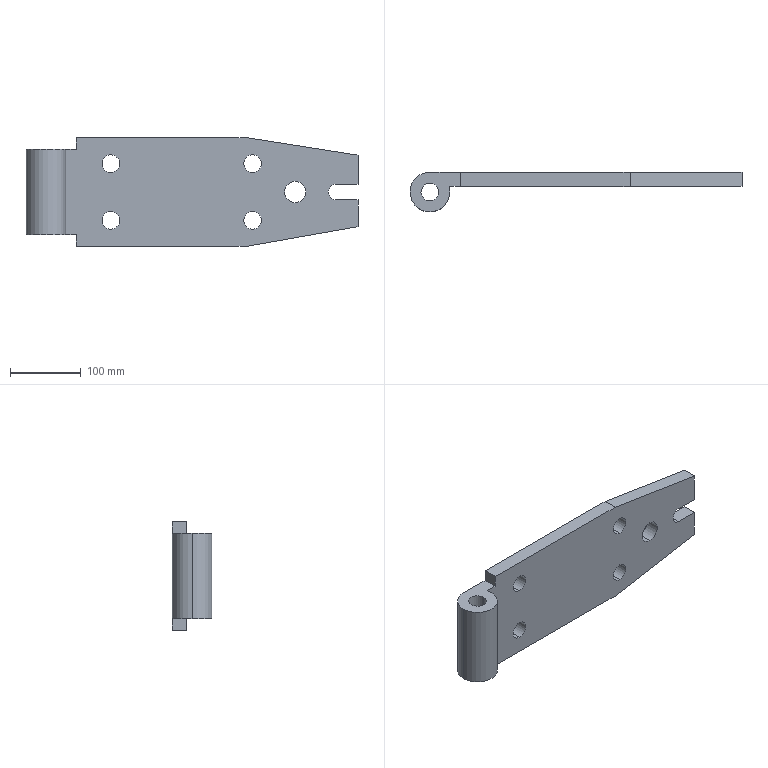Part | SolidWorks | features Extrusion 1, ICE 1 | 1 solid | 30 faces | box 468.278 x 56 x 153.374 mm | volume 1357843 mm3 | cylinder 15 | plane 15 | commonest cylinder face diameters 25 x10 30 x2 56 x2 22.074 x1
STEP:
#1=CARTESIAN_POINT('',(-212.267,-8.,60.));
#2=VERTEX_POINT('',#1);
#3=CARTESIAN_POINT('',(-187.267,-8.,60.));
#4=VERTEX_POINT('',#3);
#5=CARTESIAN_POINT('',(-199.767,-8.,60.));
#6=DIRECTION('',(0.,0.,1.));
#7=DIRECTION('',(1.,0.,0.));
#8=AXIS2_PLACEMENT_3D('',#5,#6,#7);
#9=CIRCLE('',#8,12.5);
#10=EDGE_CURVE('',#2,#4,#9,.T.);
#11=ORIENTED_EDGE('',*,*,#10,.T.);
#12=CARTESIAN_POINT('',(-187.267,-8.,-60.));
#13=VERTEX_POINT('',#12);
#14=CARTESIAN_POINT('',(-187.267,-8.,60.));
#15=DIRECTION('',(0.,0.,-1.));
#16=VECTOR('',#15,1000.);
#17=LINE('',#14,#16);
#18=EDGE_CURVE('',#4,#13,#17,.T.);
#19=ORIENTED_EDGE('',*,*,#18,.T.);
#20=CARTESIAN_POINT('',(-212.267,-8.,-60.));
#21=VERTEX_POINT('',#20);
#22=CARTESIAN_POINT('',(-199.767,-8.,-60.));
#23=DIRECTION('',(0.,0.,1.));
#24=DIRECTION('',(1.,0.,0.));
#25=AXIS2_PLACEMENT_3D('',#22,#23,#24);
#26=CIRCLE('',#25,12.5);
#27=EDGE_CURVE('',#21,#13,#26,.T.);
#28=ORIENTED_EDGE('',*,*,#27,.F.);
#29=CARTESIAN_POINT('',(-212.267,-8.,60.));
#30=DIRECTION('',(0.,0.,-1.));
#31=VECTOR('',#30,1000.);
#32=LINE('',#29,#31);
#33=EDGE_CURVE('',#2,#21,#32,.T.);
#34=ORIENTED_EDGE('',*,*,#33,.F.);
#35=EDGE_LOOP('',(#11,#19,#28,#34));
#36=FACE_OUTER_BOUND('',#35,.T.);
#37=CARTESIAN_POINT('',(-199.767,-8.,60.));
#38=DIRECTION('',(0.,0.,-1.));
#39=DIRECTION('',(-1.,0.,0.));
#40=AXIS2_PLACEMENT_3D('',#37,#38,#39);
#41=CYLINDRICAL_SURFACE('',#40,12.5);
#42=ADVANCED_FACE('',(#36),#41,.F.);
#43=CARTESIAN_POINT('',(-227.767,-8.,60.));
#44=VERTEX_POINT('',#43);
#45=CARTESIAN_POINT('',(-171.767,-8.,60.));
#46=VERTEX_POINT('',#45);
#47=CARTESIAN_POINT('',(-199.767,-8.,60.));
#48=DIRECTION('',(0.,0.,1.));
#49=DIRECTION('',(1.,0.,0.));
#50=AXIS2_PLACEMENT_3D('',#47,#48,#49);
#51=CIRCLE('',#50,28.);
#52=EDGE_CURVE('',#44,#46,#51,.T.);
#53=ORIENTED_EDGE('',*,*,#52,.F.);
#54=CARTESIAN_POINT('',(-227.767,-8.,-60.));
#55=VERTEX_POINT('',#54);
#56=CARTESIAN_POINT('',(-227.767,-8.,60.));
#57=DIRECTION('',(0.,0.,-1.));
#58=VECTOR('',#57,1000.);
#59=LINE('',#56,#58);
#60=EDGE_CURVE('',#44,#55,#59,.T.);
#61=ORIENTED_EDGE('',*,*,#60,.T.);
#62=CARTESIAN_POINT('',(-171.767,-8.,-60.));
#63=VERTEX_POINT('',#62);
#64=CARTESIAN_POINT('',(-199.767,-8.,-60.));
#65=DIRECTION('',(0.,0.,1.));
#66=DIRECTION('',(1.,0.,0.));
#67=AXIS2_PLACEMENT_3D('',#64,#65,#66);
#68=CIRCLE('',#67,28.);
#69=EDGE_CURVE('',#55,#63,#68,.T.);
#70=ORIENTED_EDGE('',*,*,#69,.T.);
#71=CARTESIAN_POINT('',(-171.767,-8.,60.));
#72=DIRECTION('',(0.,0.,-1.));
#73=VECTOR('',#72,1000.);
#74=LINE('',#71,#73);
#75=EDGE_CURVE('',#46,#63,#74,.T.);
#76=ORIENTED_EDGE('',*,*,#75,.F.);
#77=EDGE_LOOP('',(#53,#61,#70,#76));
#78=FACE_OUTER_BOUND('',#77,.T.);
#79=CARTESIAN_POINT('',(-199.767,-8.,60.));
#80=DIRECTION('',(0.,0.,-1.));
#81=DIRECTION('',(-1.,0.,0.));
#82=AXIS2_PLACEMENT_3D('',#79,#80,#81);
#83=CYLINDRICAL_SURFACE('',#82,28.);
#84=ADVANCED_FACE('',(#78),#83,.T.);
#85=CARTESIAN_POINT('',(-108.15,20.,27.5));
#86=VERTEX_POINT('',#85);
#87=CARTESIAN_POINT('',(-108.15,20.,52.5));
#88=VERTEX_POINT('',#87);
#89=CARTESIAN_POINT('',(-108.15,20.,40.));
#90=DIRECTION('',(0.,1.,0.));
#91=DIRECTION('',(0.,0.,1.));
#92=AXIS2_PLACEMENT_3D('',#89,#90,#91);
#93=CIRCLE('',#92,12.5);
#94=EDGE_CURVE('',#86,#88,#93,.T.);
#95=ORIENTED_EDGE('',*,*,#94,.T.);
#96=CARTESIAN_POINT('',(-108.15,0.,52.5));
#97=VERTEX_POINT('',#96);
#98=CARTESIAN_POINT('',(-108.15,20.,52.5));
#99=DIRECTION('',(0.,-1.,0.));
#100=VECTOR('',#99,1000.);
#101=LINE('',#98,#100);
#102=EDGE_CURVE('',#88,#97,#101,.T.);
#103=ORIENTED_EDGE('',*,*,#102,.T.);
#104=CARTESIAN_POINT('',(-108.15,0.,27.5));
#105=VERTEX_POINT('',#104);
#106=CARTESIAN_POINT('',(-108.15,0.,40.));
#107=DIRECTION('',(0.,1.,0.));
#108=DIRECTION('',(0.,0.,1.));
#109=AXIS2_PLACEMENT_3D('',#106,#107,#108);
#110=CIRCLE('',#109,12.5);
#111=EDGE_CURVE('',#105,#97,#110,.T.);
#112=ORIENTED_EDGE('',*,*,#111,.F.);
#113=CARTESIAN_POINT('',(-108.15,20.,27.5));
#114=DIRECTION('',(0.,-1.,0.));
#115=VECTOR('',#114,1000.);
#116=LINE('',#113,#115);
#117=EDGE_CURVE('',#86,#105,#116,.T.);
#118=ORIENTED_EDGE('',*,*,#117,.F.);
#119=EDGE_LOOP('',(#95,#103,#112,#118));
#120=FACE_OUTER_BOUND('',#119,.T.);
#121=CARTESIAN_POINT('',(-108.15,20.,40.));
#122=DIRECTION('',(0.,-1.,0.));
#123=DIRECTION('',(0.,0.,-1.));
#124=AXIS2_PLACEMENT_3D('',#121,#122,#123);
#125=CYLINDRICAL_SURFACE('',#124,12.5);
#126=ADVANCED_FACE('',(#120),#125,.F.);
#127=CARTESIAN_POINT('',(91.85,20.,27.5));
#128=VERTEX_POINT('',#127);
#129=CARTESIAN_POINT('',(91.85,20.,52.5));
#130=VERTEX_POINT('',#129);
#131=CARTESIAN_POINT('',(91.85,20.,40.));
#132=DIRECTION('',(0.,1.,0.));
#133=DIRECTION('',(0.,0.,1.));
#134=AXIS2_PLACEMENT_3D('',#131,#132,#133);
#135=CIRCLE('',#134,12.5);
#136=EDGE_CURVE('',#128,#130,#135,.T.);
#137=ORIENTED_EDGE('',*,*,#136,.T.);
#138=CARTESIAN_POINT('',(91.85,0.,52.5));
#139=VERTEX_POINT('',#138);
#140=CARTESIAN_POINT('',(91.85,20.,52.5));
#141=DIRECTION('',(0.,-1.,0.));
#142=VECTOR('',#141,1000.);
#143=LINE('',#140,#142);
#144=EDGE_CURVE('',#130,#139,#143,.T.);
#145=ORIENTED_EDGE('',*,*,#144,.T.);
#146=CARTESIAN_POINT('',(91.85,0.,27.5));
#147=VERTEX_POINT('',#146);
#148=CARTESIAN_POINT('',(91.85,0.,40.));
#149=DIRECTION('',(0.,1.,0.));
#150=DIRECTION('',(0.,0.,1.));
#151=AXIS2_PLACEMENT_3D('',#148,#149,#150);
#152=CIRCLE('',#151,12.5);
#153=EDGE_CURVE('',#147,#139,#152,.T.);
#154=ORIENTED_EDGE('',*,*,#153,.F.);
#155=CARTESIAN_POINT('',(91.85,20.,27.5));
#156=DIRECTION('',(0.,-1.,0.));
#157=VECTOR('',#156,1000.);
#158=LINE('',#155,#157);
#159=EDGE_CURVE('',#128,#147,#158,.T.);
#160=ORIENTED_EDGE('',*,*,#159,.F.);
#161=EDGE_LOOP('',(#137,#145,#154,#160));
#162=FACE_OUTER_BOUND('',#161,.T.);
#163=CARTESIAN_POINT('',(91.85,20.,40.));
#164=DIRECTION('',(0.,-1.,0.));
#165=DIRECTION('',(0.,0.,-1.));
#166=AXIS2_PLACEMENT_3D('',#163,#164,#165);
#167=CYLINDRICAL_SURFACE('',#166,12.5);
#168=ADVANCED_FACE('',(#162),#167,.F.);
#169=CARTESIAN_POINT('',(151.85,20.,-15.));
#170=VERTEX_POINT('',#169);
#171=CARTESIAN_POINT('',(151.85,20.,15.));
#172=VERTEX_POINT('',#171);
#173=CARTESIAN_POINT('',(151.85,20.,0.));
#174=DIRECTION('',(0.,1.,0.));
#175=DIRECTION('',(0.,0.,1.));
#176=AXIS2_PLACEMENT_3D('',#173,#174,#175);
#177=CIRCLE('',#176,15.);
#178=EDGE_CURVE('',#170,#172,#177,.T.);
#179=ORIENTED_EDGE('',*,*,#178,.T.);
#180=CARTESIAN_POINT('',(151.85,0.,15.));
#181=VERTEX_POINT('',#180);
#182=CARTESIAN_POINT('',(151.85,20.,15.));
#183=DIRECTION('',(0.,-1.,0.));
#184=VECTOR('',#183,1000.);
#185=LINE('',#182,#184);
#186=EDGE_CURVE('',#172,#181,#185,.T.);
#187=ORIENTED_EDGE('',*,*,#186,.T.);
#188=CARTESIAN_POINT('',(151.85,0.,-15.));
#189=VERTEX_POINT('',#188);
#190=CARTESIAN_POINT('',(151.85,0.,0.));
#191=DIRECTION('',(0.,1.,0.));
#192=DIRECTION('',(0.,0.,1.));
#193=AXIS2_PLACEMENT_3D('',#190,#191,#192);
#194=CIRCLE('',#193,15.);
#195=EDGE_CURVE('',#189,#181,#194,.T.);
#196=ORIENTED_EDGE('',*,*,#195,.F.);
#197=CARTESIAN_POINT('',(151.85,20.,-15.));
#198=DIRECTION('',(0.,-1.,0.));
#199=VECTOR('',#198,1000.);
#200=LINE('',#197,#199);
#201=EDGE_CURVE('',#170,#189,#200,.T.);
#202=ORIENTED_EDGE('',*,*,#201,.F.);
#203=EDGE_LOOP('',(#179,#187,#196,#202));
#204=FACE_OUTER_BOUND('',#203,.T.);
#205=CARTESIAN_POINT('',(151.85,20.,0.));
#206=DIRECTION('',(0.,-1.,0.));
#207=DIRECTION('',(0.,0.,-1.));
#208=AXIS2_PLACEMENT_3D('',#205,#206,#207);
#209=CYLINDRICAL_SURFACE('',#208,15.);
#210=ADVANCED_FACE('',(#204),#209,.F.);
#211=CARTESIAN_POINT('',(-108.15,20.,-52.5));
#212=VERTEX_POINT('',#211);
#213=CARTESIAN_POINT('',(-108.15,20.,-27.5));
#214=VERTEX_POINT('',#213);
#215=CARTESIAN_POINT('',(-108.15,20.,-40.));
#216=DIRECTION('',(0.,1.,0.));
#217=DIRECTION('',(0.,0.,1.));
#218=AXIS2_PLACEMENT_3D('',#215,#216,#217);
#219=CIRCLE('',#218,12.5);
#220=EDGE_CURVE('',#212,#214,#219,.T.);
#221=ORIENTED_EDGE('',*,*,#220,.T.);
#222=CARTESIAN_POINT('',(-108.15,0.,-27.5));
#223=VERTEX_POINT('',#222);
#224=CARTESIAN_POINT('',(-108.15,20.,-27.5));
#225=DIRECTION('',(0.,-1.,0.));
#226=VECTOR('',#225,1000.);
#227=LINE('',#224,#226);
#228=EDGE_CURVE('',#214,#223,#227,.T.);
#229=ORIENTED_EDGE('',*,*,#228,.T.);
#230=CARTESIAN_POINT('',(-108.15,0.,-52.5));
#231=VERTEX_POINT('',#230);
#232=CARTESIAN_POINT('',(-108.15,0.,-40.));
#233=DIRECTION('',(0.,1.,0.));
#234=DIRECTION('',(0.,0.,1.));
#235=AXIS2_PLACEMENT_3D('',#232,#233,#234);
#236=CIRCLE('',#235,12.5);
#237=EDGE_CURVE('',#231,#223,#236,.T.);
#238=ORIENTED_EDGE('',*,*,#237,.F.);
#239=CARTESIAN_POINT('',(-108.15,20.,-52.5));
#240=DIRECTION('',(0.,-1.,0.));
#241=VECTOR('',#240,1000.);
#242=LINE('',#239,#241);
#243=EDGE_CURVE('',#212,#231,#242,.T.);
#244=ORIENTED_EDGE('',*,*,#243,.F.);
#245=EDGE_LOOP('',(#221,#229,#238,#244));
#246=FACE_OUTER_BOUND('',#245,.T.);
#247=CARTESIAN_POINT('',(-108.15,20.,-40.));
#248=DIRECTION('',(0.,-1.,0.));
#249=DIRECTION('',(0.,0.,-1.));
#250=AXIS2_PLACEMENT_3D('',#247,#248,#249);
#251=CYLINDRICAL_SURFACE('',#250,12.5);
#252=ADVANCED_FACE('',(#246),#251,.F.);
#253=CARTESIAN_POINT('',(91.85,20.,-52.5));
#254=VERTEX_POINT('',#253);
#255=CARTESIAN_POINT('',(91.85,20.,-27.5));
#256=VERTEX_POINT('',#255);
#257=CARTESIAN_POINT('',(91.85,20.,-40.));
#258=DIRECTION('',(0.,1.,0.));
#259=DIRECTION('',(0.,0.,1.));
#260=AXIS2_PLACEMENT_3D('',#257,#258,#259);
#261=CIRCLE('',#260,12.5);
#262=EDGE_CURVE('',#254,#256,#261,.T.);
#263=ORIENTED_EDGE('',*,*,#262,.T.);
#264=CARTESIAN_POINT('',(91.85,0.,-27.5));
#265=VERTEX_POINT('',#264);
#266=CARTESIAN_POINT('',(91.85,20.,-27.5));
#267=DIRECTION('',(0.,-1.,0.));
#268=VECTOR('',#267,1000.);
#269=LINE('',#266,#268);
#270=EDGE_CURVE('',#256,#265,#269,.T.);
#271=ORIENTED_EDGE('',*,*,#270,.T.);
#272=CARTESIAN_POINT('',(91.85,0.,-52.5));
#273=VERTEX_POINT('',#272);
#274=CARTESIAN_POINT('',(91.85,0.,-40.));
#275=DIRECTION('',(0.,1.,0.));
#276=DIRECTION('',(0.,0.,1.));
#277=AXIS2_PLACEMENT_3D('',#274,#275,#276);
#278=CIRCLE('',#277,12.5);
#279=EDGE_CURVE('',#273,#265,#278,.T.);
#280=ORIENTED_EDGE('',*,*,#279,.F.);
#281=CARTESIAN_POINT('',(91.85,20.,-52.5));
#282=DIRECTION('',(0.,-1.,0.));
#283=VECTOR('',#282,1000.);
#284=LINE('',#281,#283);
#285=EDGE_CURVE('',#254,#273,#284,.T.);
#286=ORIENTED_EDGE('',*,*,#285,.F.);
#287=EDGE_LOOP('',(#263,#271,#280,#286));
#288=FACE_OUTER_BOUND('',#287,.T.);
#289=CARTESIAN_POINT('',(91.85,20.,-40.));
#290=DIRECTION('',(0.,-1.,0.));
#291=DIRECTION('',(0.,0.,-1.));
#292=AXIS2_PLACEMENT_3D('',#289,#290,#291);
#293=CYLINDRICAL_SURFACE('',#292,12.5);
#294=ADVANCED_FACE('',(#288),#293,.F.);
#295=CARTESIAN_POINT('',(-156.767,0.,76.687));
#296=VERTEX_POINT('',#295);
#297=CARTESIAN_POINT('',(82.575,0.,76.687));
#298=VERTEX_POINT('',#297);
#299=CARTESIAN_POINT('',(0.,0.,76.687));
#300=DIRECTION('',(1.,0.,0.));
#301=VECTOR('',#300,1000.);
#302=LINE('',#299,#301);
#303=EDGE_CURVE('',#296,#298,#302,.T.);
#304=ORIENTED_EDGE('',*,*,#303,.T.);
#305=CARTESIAN_POINT('',(82.575,20.,76.687));
#306=VERTEX_POINT('',#305);
#307=CARTESIAN_POINT('',(82.575,20.,76.687));
#308=DIRECTION('',(0.,-1.,0.));
#309=VECTOR('',#308,1000.);
#310=LINE('',#307,#309);
#311=EDGE_CURVE('',#306,#298,#310,.T.);
#312=ORIENTED_EDGE('',*,*,#311,.F.);
#313=CARTESIAN_POINT('',(-156.767,20.,76.687));
#314=VERTEX_POINT('',#313);
#315=CARTESIAN_POINT('',(0.,20.,76.687));
#316=DIRECTION('',(1.,0.,0.));
#317=VECTOR('',#316,1000.);
#318=LINE('',#315,#317);
#319=EDGE_CURVE('',#314,#306,#318,.T.);
#320=ORIENTED_EDGE('',*,*,#319,.F.);
#321=CARTESIAN_POINT('',(-156.767,20.,76.687));
#322=DIRECTION('',(0.,-1.,0.));
#323=VECTOR('',#322,1000.);
#324=LINE('',#321,#323);
#325=EDGE_CURVE('',#314,#296,#324,.T.);
#326=ORIENTED_EDGE('',*,*,#325,.T.);
#327=EDGE_LOOP('',(#304,#312,#320,#326));
#328=FACE_OUTER_BOUND('',#327,.T.);
#329=CARTESIAN_POINT('',(0.,20.,76.687));
#330=DIRECTION('',(0.,0.,-1.));
#331=DIRECTION('',(-1.,0.,0.));
#332=AXIS2_PLACEMENT_3D('',#329,#330,#331);
#333=PLANE('',#332);
#334=ADVANCED_FACE('',(#328),#333,.F.);
#335=CARTESIAN_POINT('',(240.511,0.,51.991));
#336=VERTEX_POINT('',#335);
#337=CARTESIAN_POINT('',(13.676,0.,87.461));
#338=DIRECTION('',(0.988,0.,-0.1545));
#339=VECTOR('',#338,1000.);
#340=LINE('',#337,#339);
#341=EDGE_CURVE('',#298,#336,#340,.T.);
#342=ORIENTED_EDGE('',*,*,#341,.T.);
#343=CARTESIAN_POINT('',(240.511,20.,51.991));
#344=VERTEX_POINT('',#343);
#345=CARTESIAN_POINT('',(240.511,20.,51.991));
#346=DIRECTION('',(0.,-1.,0.));
#347=VECTOR('',#346,1000.);
#348=LINE('',#345,#347);
#349=EDGE_CURVE('',#344,#336,#348,.T.);
#350=ORIENTED_EDGE('',*,*,#349,.F.);
#351=CARTESIAN_POINT('',(13.676,20.,87.461));
#352=DIRECTION('',(0.988,0.,-0.1545));
#353=VECTOR('',#352,1000.);
#354=LINE('',#351,#353);
#355=EDGE_CURVE('',#306,#344,#354,.T.);
#356=ORIENTED_EDGE('',*,*,#355,.F.);
#357=ORIENTED_EDGE('',*,*,#311,.T.);
#358=EDGE_LOOP('',(#342,#350,#356,#357));
#359=FACE_OUTER_BOUND('',#358,.T.);
#360=CARTESIAN_POINT('',(13.676,20.,87.461));
#361=DIRECTION('',(-0.1545,0.,-0.988));
#362=DIRECTION('',(-0.988,0.,0.1545));
#363=AXIS2_PLACEMENT_3D('',#360,#361,#362);
#364=PLANE('',#363);
#365=ADVANCED_FACE('',(#359),#364,.F.);
#366=CARTESIAN_POINT('',(240.511,0.,11.));
#367=VERTEX_POINT('',#366);
#368=CARTESIAN_POINT('',(240.511,0.,0.));
#369=DIRECTION('',(0.,0.,1.));
#370=VECTOR('',#369,1000.);
#371=LINE('',#368,#370);
#372=EDGE_CURVE('',#367,#336,#371,.T.);
#373=ORIENTED_EDGE('',*,*,#372,.F.);
#374=CARTESIAN_POINT('',(240.511,20.,11.));
#375=VERTEX_POINT('',#374);
#376=CARTESIAN_POINT('',(240.511,20.,11.));
#377=DIRECTION('',(0.,-1.,0.));
#378=VECTOR('',#377,1000.);
#379=LINE('',#376,#378);
#380=EDGE_CURVE('',#375,#367,#379,.T.);
#381=ORIENTED_EDGE('',*,*,#380,.F.);
#382=CARTESIAN_POINT('',(240.511,20.,0.));
#383=DIRECTION('',(0.,0.,1.));
#384=VECTOR('',#383,1000.);
#385=LINE('',#382,#384);
#386=EDGE_CURVE('',#375,#344,#385,.T.);
#387=ORIENTED_EDGE('',*,*,#386,.T.);
#388=ORIENTED_EDGE('',*,*,#349,.T.);
#389=EDGE_LOOP('',(#373,#381,#387,#388));
#390=FACE_OUTER_BOUND('',#389,.T.);
#391=CARTESIAN_POINT('',(240.511,20.,0.));
#392=DIRECTION('',(1.,0.,0.));
#393=DIRECTION('',(0.,0.,-1.));
#394=AXIS2_PLACEMENT_3D('',#391,#392,#393);
#395=PLANE('',#394);
#396=ADVANCED_FACE('',(#390),#395,.T.);
#397=CARTESIAN_POINT('',(208.511,0.,11.));
#398=VERTEX_POINT('',#397);
#399=CARTESIAN_POINT('',(0.,0.,11.));
#400=DIRECTION('',(-1.,0.,0.));
#401=VECTOR('',#400,1000.);
#402=LINE('',#399,#401);
#403=EDGE_CURVE('',#367,#398,#402,.T.);
#404=ORIENTED_EDGE('',*,*,#403,.T.);
#405=CARTESIAN_POINT('',(208.511,20.,11.));
#406=VERTEX_POINT('',#405);
#407=CARTESIAN_POINT('',(208.511,20.,11.));
#408=DIRECTION('',(0.,-1.,0.));
#409=VECTOR('',#408,1000.);
#410=LINE('',#407,#409);
#411=EDGE_CURVE('',#406,#398,#410,.T.);
#412=ORIENTED_EDGE('',*,*,#411,.F.);
#413=CARTESIAN_POINT('',(0.,20.,11.));
#414=DIRECTION('',(-1.,0.,0.));
#415=VECTOR('',#414,1000.);
#416=LINE('',#413,#415);
#417=EDGE_CURVE('',#375,#406,#416,.T.);
#418=ORIENTED_EDGE('',*,*,#417,.F.);
#419=ORIENTED_EDGE('',*,*,#380,.T.);
#420=EDGE_LOOP('',(#404,#412,#418,#419));
#421=FACE_OUTER_BOUND('',#420,.T.);
#422=CARTESIAN_POINT('',(0.,20.,11.));
#423=DIRECTION('',(0.,0.,1.));
#424=DIRECTION('',(1.,0.,0.));
#425=AXIS2_PLACEMENT_3D('',#422,#423,#424);
#426=PLANE('',#425);
#427=ADVANCED_FACE('',(#421),#426,.F.);
#428=CARTESIAN_POINT('',(208.511,0.,-11.));
#429=VERTEX_POINT('',#428);
#430=CARTESIAN_POINT('',(209.414,0.,0.));
#431=DIRECTION('',(0.,1.,0.));
#432=DIRECTION('',(0.,0.,1.));
#433=AXIS2_PLACEMENT_3D('',#430,#431,#432);
#434=CIRCLE('',#433,11.037);
#435=EDGE_CURVE('',#429,#398,#434,.T.);
#436=ORIENTED_EDGE('',*,*,#435,.F.);
#437=CARTESIAN_POINT('',(208.511,20.,-11.));
#438=VERTEX_POINT('',#437);
#439=CARTESIAN_POINT('',(208.511,20.,-11.));
#440=DIRECTION('',(0.,-1.,0.));
#441=VECTOR('',#440,1000.);
#442=LINE('',#439,#441);
#443=EDGE_CURVE('',#438,#429,#442,.T.);
#444=ORIENTED_EDGE('',*,*,#443,.F.);
#445=CARTESIAN_POINT('',(209.414,20.,0.));
#446=DIRECTION('',(0.,1.,0.));
#447=DIRECTION('',(0.,0.,1.));
#448=AXIS2_PLACEMENT_3D('',#445,#446,#447);
#449=CIRCLE('',#448,11.037);
#450=EDGE_CURVE('',#438,#406,#449,.T.);
#451=ORIENTED_EDGE('',*,*,#450,.T.);
#452=ORIENTED_EDGE('',*,*,#411,.T.);
#453=EDGE_LOOP('',(#436,#444,#451,#452));
#454=FACE_OUTER_BOUND('',#453,.T.);
#455=CARTESIAN_POINT('',(209.414,20.,0.));
#456=DIRECTION('',(0.,-1.,0.));
#457=DIRECTION('',(0.,0.,-1.));
#458=AXIS2_PLACEMENT_3D('',#455,#456,#457);
#459=CYLINDRICAL_SURFACE('',#458,11.037);
#460=ADVANCED_FACE('',(#454),#459,.F.);
#461=CARTESIAN_POINT('',(240.511,0.,-11.));
#462=VERTEX_POINT('',#461);
#463=CARTESIAN_POINT('',(0.,0.,-11.));
#464=DIRECTION('',(-1.,0.,0.));
#465=VECTOR('',#464,1000.);
#466=LINE('',#463,#465);
#467=EDGE_CURVE('',#462,#429,#466,.T.);
#468=ORIENTED_EDGE('',*,*,#467,.F.);
#469=CARTESIAN_POINT('',(240.511,20.,-11.));
#470=VERTEX_POINT('',#469);
#471=CARTESIAN_POINT('',(240.511,20.,-11.));
#472=DIRECTION('',(0.,-1.,0.));
#473=VECTOR('',#472,1000.);
#474=LINE('',#471,#473);
#475=EDGE_CURVE('',#470,#462,#474,.T.);
#476=ORIENTED_EDGE('',*,*,#475,.F.);
#477=CARTESIAN_POINT('',(0.,20.,-11.));
#478=DIRECTION('',(-1.,0.,0.));
#479=VECTOR('',#478,1000.);
#480=LINE('',#477,#479);
#481=EDGE_CURVE('',#470,#438,#480,.T.);
#482=ORIENTED_EDGE('',*,*,#481,.T.);
#483=ORIENTED_EDGE('',*,*,#443,.T.);
#484=EDGE_LOOP('',(#468,#476,#482,#483));
#485=FACE_OUTER_BOUND('',#484,.T.);
#486=CARTESIAN_POINT('',(0.,20.,-11.));
#487=DIRECTION('',(0.,0.,1.));
#488=DIRECTION('',(1.,0.,0.));
#489=AXIS2_PLACEMENT_3D('',#486,#487,#488);
#490=PLANE('',#489);
#491=ADVANCED_FACE('',(#485),#490,.T.);
#492=CARTESIAN_POINT('',(240.511,0.,-49.));
#493=VERTEX_POINT('',#492);
#494=CARTESIAN_POINT('',(240.511,0.,0.));
#495=DIRECTION('',(0.,0.,1.));
#496=VECTOR('',#495,1000.);
#497=LINE('',#494,#496);
#498=EDGE_CURVE('',#493,#462,#497,.T.);
#499=ORIENTED_EDGE('',*,*,#498,.F.);
#500=CARTESIAN_POINT('',(240.511,20.,-49.));
#501=VERTEX_POINT('',#500);
#502=CARTESIAN_POINT('',(240.511,20.,-49.));
#503=DIRECTION('',(0.,-1.,0.));
#504=VECTOR('',#503,1000.);
#505=LINE('',#502,#504);
#506=EDGE_CURVE('',#501,#493,#505,.T.);
#507=ORIENTED_EDGE('',*,*,#506,.F.);
#508=CARTESIAN_POINT('',(240.511,20.,0.));
#509=DIRECTION('',(0.,0.,1.));
#510=VECTOR('',#509,1000.);
#511=LINE('',#508,#510);
#512=EDGE_CURVE('',#501,#470,#511,.T.);
#513=ORIENTED_EDGE('',*,*,#512,.T.);
#514=ORIENTED_EDGE('',*,*,#475,.T.);
#515=EDGE_LOOP('',(#499,#507,#513,#514));
#516=FACE_OUTER_BOUND('',#515,.T.);
#517=CARTESIAN_POINT('',(240.511,20.,0.));
#518=DIRECTION('',(1.,0.,0.));
#519=DIRECTION('',(0.,0.,-1.));
#520=AXIS2_PLACEMENT_3D('',#517,#518,#519);
#521=PLANE('',#520);
#522=ADVANCED_FACE('',(#516),#521,.T.);
#523=CARTESIAN_POINT('',(82.575,0.,-76.687));
#524=VERTEX_POINT('',#523);
#525=CARTESIAN_POINT('',(15.505,0.,-88.445));
#526=DIRECTION('',(0.985,0.,0.1727));
#527=VECTOR('',#526,1000.);
#528=LINE('',#525,#527);
#529=EDGE_CURVE('',#524,#493,#528,.T.);
#530=ORIENTED_EDGE('',*,*,#529,.F.);
#531=CARTESIAN_POINT('',(82.575,20.,-76.687));
#532=VERTEX_POINT('',#531);
#533=CARTESIAN_POINT('',(82.575,20.,-76.687));
#534=DIRECTION('',(0.,-1.,0.));
#535=VECTOR('',#534,1000.);
#536=LINE('',#533,#535);
#537=EDGE_CURVE('',#532,#524,#536,.T.);
#538=ORIENTED_EDGE('',*,*,#537,.F.);
#539=CARTESIAN_POINT('',(15.505,20.,-88.445));
#540=DIRECTION('',(0.985,0.,0.1727));
#541=VECTOR('',#540,1000.);
#542=LINE('',#539,#541);
#543=EDGE_CURVE('',#532,#501,#542,.T.);
#544=ORIENTED_EDGE('',*,*,#543,.T.);
#545=ORIENTED_EDGE('',*,*,#506,.T.);
#546=EDGE_LOOP('',(#530,#538,#544,#545));
#547=FACE_OUTER_BOUND('',#546,.T.);
#548=CARTESIAN_POINT('',(15.505,20.,-88.445));
#549=DIRECTION('',(0.1727,0.,-0.985));
#550=DIRECTION('',(-0.985,0.,-0.1727));
#551=AXIS2_PLACEMENT_3D('',#548,#549,#550);
#552=PLANE('',#551);
#553=ADVANCED_FACE('',(#547),#552,.T.);
#554=CARTESIAN_POINT('',(-156.767,0.,-76.687));
#555=VERTEX_POINT('',#554);
#556=CARTESIAN_POINT('',(0.,0.,-76.687));
#557=DIRECTION('',(1.,0.,0.));
#558=VECTOR('',#557,1000.);
#559=LINE('',#556,#558);
#560=EDGE_CURVE('',#555,#524,#559,.T.);
#561=ORIENTED_EDGE('',*,*,#560,.F.);
#562=CARTESIAN_POINT('',(-156.767,20.,-76.687));
#563=VERTEX_POINT('',#562);
#564=CARTESIAN_POINT('',(-156.767,20.,-76.687));
#565=DIRECTION('',(0.,-1.,0.));
#566=VECTOR('',#565,1000.);
#567=LINE('',#564,#566);
#568=EDGE_CURVE('',#563,#555,#567,.T.);
#569=ORIENTED_EDGE('',*,*,#568,.F.);
#570=CARTESIAN_POINT('',(0.,20.,-76.687));
#571=DIRECTION('',(1.,0.,0.));
#572=VECTOR('',#571,1000.);
#573=LINE('',#570,#572);
#574=EDGE_CURVE('',#563,#532,#573,.T.);
#575=ORIENTED_EDGE('',*,*,#574,.T.);
#576=ORIENTED_EDGE('',*,*,#537,.T.);
#577=EDGE_LOOP('',(#561,#569,#575,#576));
#578=FACE_OUTER_BOUND('',#577,.T.);
#579=CARTESIAN_POINT('',(0.,20.,-76.687));
#580=DIRECTION('',(0.,0.,-1.));
#581=DIRECTION('',(-1.,0.,0.));
#582=AXIS2_PLACEMENT_3D('',#579,#580,#581);
#583=PLANE('',#582);
#584=ADVANCED_FACE('',(#578),#583,.T.);
#585=CARTESIAN_POINT('',(-156.767,0.,-60.));
#586=VERTEX_POINT('',#585);
#587=CARTESIAN_POINT('',(-156.767,0.,0.));
#588=DIRECTION('',(0.,0.,-1.));
#589=VECTOR('',#588,1000.);
#590=LINE('',#587,#589);
#591=EDGE_CURVE('',#586,#555,#590,.T.);
#592=ORIENTED_EDGE('',*,*,#591,.F.);
#593=CARTESIAN_POINT('',(-156.767,20.,-60.));
#594=VERTEX_POINT('',#593);
#595=CARTESIAN_POINT('',(-156.767,20.,-60.));
#596=DIRECTION('',(0.,-1.,0.));
#597=VECTOR('',#596,1000.);
#598=LINE('',#595,#597);
#599=EDGE_CURVE('',#594,#586,#598,.T.);
#600=ORIENTED_EDGE('',*,*,#599,.F.);
#601=CARTESIAN_POINT('',(-156.767,20.,0.));
#602=DIRECTION('',(0.,0.,-1.));
#603=VECTOR('',#602,1000.);
#604=LINE('',#601,#603);
#605=EDGE_CURVE('',#594,#563,#604,.T.);
#606=ORIENTED_EDGE('',*,*,#605,.T.);
#607=ORIENTED_EDGE('',*,*,#568,.T.);
#608=EDGE_LOOP('',(#592,#600,#606,#607));
#609=FACE_OUTER_BOUND('',#608,.T.);
#610=CARTESIAN_POINT('',(-156.767,20.,0.));
#611=DIRECTION('',(-1.,0.,0.));
#612=DIRECTION('',(0.,0.,1.));
#613=AXIS2_PLACEMENT_3D('',#610,#611,#612);
#614=PLANE('',#613);
#615=ADVANCED_FACE('',(#609),#614,.T.);
#616=CARTESIAN_POINT('',(-171.767,0.,-60.));
#617=VERTEX_POINT('',#616);
#618=CARTESIAN_POINT('',(0.,0.,-60.));
#619=DIRECTION('',(1.,0.,0.));
#620=VECTOR('',#619,1000.);
#621=LINE('',#618,#620);
#622=EDGE_CURVE('',#617,#586,#621,.T.);
#623=ORIENTED_EDGE('',*,*,#622,.F.);
#624=CARTESIAN_POINT('',(-171.767,0.,-60.));
#625=DIRECTION('',(0.,-1.,0.));
#626=VECTOR('',#625,1000.);
#627=LINE('',#624,#626);
#628=EDGE_CURVE('',#617,#63,#627,.T.);
#629=ORIENTED_EDGE('',*,*,#628,.T.);
#630=ORIENTED_EDGE('',*,*,#69,.F.);
#631=CARTESIAN_POINT('',(-199.767,20.,-60.));
#632=VERTEX_POINT('',#631);
#633=CARTESIAN_POINT('',(-199.767,-8.,-60.));
#634=DIRECTION('',(0.,0.,1.));
#635=DIRECTION('',(1.,0.,0.));
#636=AXIS2_PLACEMENT_3D('',#633,#634,#635);
#637=CIRCLE('',#636,28.);
#638=EDGE_CURVE('',#632,#55,#637,.T.);
#639=ORIENTED_EDGE('',*,*,#638,.F.);
#640=CARTESIAN_POINT('',(0.,20.,-60.));
#641=DIRECTION('',(1.,0.,0.));
#642=VECTOR('',#641,1000.);
#643=LINE('',#640,#642);
#644=EDGE_CURVE('',#632,#594,#643,.T.);
#645=ORIENTED_EDGE('',*,*,#644,.T.);
#646=ORIENTED_EDGE('',*,*,#599,.T.);
#647=EDGE_LOOP('',(#623,#629,#630,#639,#645,#646));
#648=FACE_OUTER_BOUND('',#647,.T.);
#649=ORIENTED_EDGE('',*,*,#27,.T.);
#650=CARTESIAN_POINT('',(-199.767,-8.,-60.));
#651=DIRECTION('',(0.,0.,1.));
#652=DIRECTION('',(1.,0.,0.));
#653=AXIS2_PLACEMENT_3D('',#650,#651,#652);
#654=CIRCLE('',#653,12.5);
#655=EDGE_CURVE('',#13,#21,#654,.T.);
#656=ORIENTED_EDGE('',*,*,#655,.T.);
#657=EDGE_LOOP('',(#649,#656));
#658=FACE_BOUND('',#657,.T.);
#659=CARTESIAN_POINT('',(0.,20.,-60.));
#660=DIRECTION('',(0.,0.,-1.));
#661=DIRECTION('',(-1.,0.,0.));
#662=AXIS2_PLACEMENT_3D('',#659,#660,#661);
#663=PLANE('',#662);
#664=ADVANCED_FACE('',(#648,#658),#663,.T.);
#665=CARTESIAN_POINT('',(-171.767,0.,60.));
#666=VERTEX_POINT('',#665);
#667=CARTESIAN_POINT('',(-156.767,0.,60.));
#668=VERTEX_POINT('',#667);
#669=CARTESIAN_POINT('',(0.,0.,60.));
#670=DIRECTION('',(1.,0.,0.));
#671=VECTOR('',#670,1000.);
#672=LINE('',#669,#671);
#673=EDGE_CURVE('',#666,#668,#672,.T.);
#674=ORIENTED_EDGE('',*,*,#673,.T.);
#675=CARTESIAN_POINT('',(-156.767,20.,60.));
#676=VERTEX_POINT('',#675);
#677=CARTESIAN_POINT('',(-156.767,20.,60.));
#678=DIRECTION('',(0.,-1.,0.));
#679=VECTOR('',#678,1000.);
#680=LINE('',#677,#679);
#681=EDGE_CURVE('',#676,#668,#680,.T.);
#682=ORIENTED_EDGE('',*,*,#681,.F.);
#683=CARTESIAN_POINT('',(-199.767,20.,60.));
#684=VERTEX_POINT('',#683);
#685=CARTESIAN_POINT('',(0.,20.,60.));
#686=DIRECTION('',(1.,0.,0.));
#687=VECTOR('',#686,1000.);
#688=LINE('',#685,#687);
#689=EDGE_CURVE('',#684,#676,#688,.T.);
#690=ORIENTED_EDGE('',*,*,#689,.F.);
#691=CARTESIAN_POINT('',(-199.767,-8.,60.));
#692=DIRECTION('',(0.,0.,1.));
#693=DIRECTION('',(1.,0.,0.));
#694=AXIS2_PLACEMENT_3D('',#691,#692,#693);
#695=CIRCLE('',#694,28.);
#696=EDGE_CURVE('',#684,#44,#695,.T.);
#697=ORIENTED_EDGE('',*,*,#696,.T.);
#698=ORIENTED_EDGE('',*,*,#52,.T.);
#699=CARTESIAN_POINT('',(-171.767,0.,60.));
#700=DIRECTION('',(0.,-1.,0.));
#701=VECTOR('',#700,1000.);
#702=LINE('',#699,#701);
#703=EDGE_CURVE('',#666,#46,#702,.T.);
#704=ORIENTED_EDGE('',*,*,#703,.F.);
#705=EDGE_LOOP('',(#674,#682,#690,#697,#698,#704));
#706=FACE_OUTER_BOUND('',#705,.T.);
#707=ORIENTED_EDGE('',*,*,#10,.F.);
#708=CARTESIAN_POINT('',(-199.767,-8.,60.));
#709=DIRECTION('',(0.,0.,1.));
#710=DIRECTION('',(1.,0.,0.));
#711=AXIS2_PLACEMENT_3D('',#708,#709,#710);
#712=CIRCLE('',#711,12.5);
#713=EDGE_CURVE('',#4,#2,#712,.T.);
#714=ORIENTED_EDGE('',*,*,#713,.F.);
#715=EDGE_LOOP('',(#707,#714));
#716=FACE_BOUND('',#715,.T.);
#717=CARTESIAN_POINT('',(0.,20.,60.));
#718=DIRECTION('',(0.,0.,-1.));
#719=DIRECTION('',(-1.,0.,0.));
#720=AXIS2_PLACEMENT_3D('',#717,#718,#719);
#721=PLANE('',#720);
#722=ADVANCED_FACE('',(#706,#716),#721,.F.);
#723=ORIENTED_EDGE('',*,*,#270,.F.);
#724=CARTESIAN_POINT('',(91.85,20.,-40.));
#725=DIRECTION('',(0.,1.,0.));
#726=DIRECTION('',(0.,0.,1.));
#727=AXIS2_PLACEMENT_3D('',#724,#725,#726);
#728=CIRCLE('',#727,12.5);
#729=EDGE_CURVE('',#256,#254,#728,.T.);
#730=ORIENTED_EDGE('',*,*,#729,.T.);
#731=ORIENTED_EDGE('',*,*,#285,.T.);
#732=CARTESIAN_POINT('',(91.85,0.,-40.));
#733=DIRECTION('',(0.,1.,0.));
#734=DIRECTION('',(0.,0.,1.));
#735=AXIS2_PLACEMENT_3D('',#732,#733,#734);
#736=CIRCLE('',#735,12.5);
#737=EDGE_CURVE('',#265,#273,#736,.T.);
#738=ORIENTED_EDGE('',*,*,#737,.F.);
#739=EDGE_LOOP('',(#723,#730,#731,#738));
#740=FACE_OUTER_BOUND('',#739,.T.);
#741=CARTESIAN_POINT('',(91.85,20.,-40.));
#742=DIRECTION('',(0.,-1.,0.));
#743=DIRECTION('',(0.,0.,-1.));
#744=AXIS2_PLACEMENT_3D('',#741,#742,#743);
#745=CYLINDRICAL_SURFACE('',#744,12.5);
#746=ADVANCED_FACE('',(#740),#745,.F.);
#747=ORIENTED_EDGE('',*,*,#228,.F.);
#748=CARTESIAN_POINT('',(-108.15,20.,-40.));
#749=DIRECTION('',(0.,1.,0.));
#750=DIRECTION('',(0.,0.,1.));
#751=AXIS2_PLACEMENT_3D('',#748,#749,#750);
#752=CIRCLE('',#751,12.5);
#753=EDGE_CURVE('',#214,#212,#752,.T.);
#754=ORIENTED_EDGE('',*,*,#753,.T.);
#755=ORIENTED_EDGE('',*,*,#243,.T.);
#756=CARTESIAN_POINT('',(-108.15,0.,-40.));
#757=DIRECTION('',(0.,1.,0.));
#758=DIRECTION('',(0.,0.,1.));
#759=AXIS2_PLACEMENT_3D('',#756,#757,#758);
#760=CIRCLE('',#759,12.5);
#761=EDGE_CURVE('',#223,#231,#760,.T.);
#762=ORIENTED_EDGE('',*,*,#761,.F.);
#763=EDGE_LOOP('',(#747,#754,#755,#762));
#764=FACE_OUTER_BOUND('',#763,.T.);
#765=CARTESIAN_POINT('',(-108.15,20.,-40.));
#766=DIRECTION('',(0.,-1.,0.));
#767=DIRECTION('',(0.,0.,-1.));
#768=AXIS2_PLACEMENT_3D('',#765,#766,#767);
#769=CYLINDRICAL_SURFACE('',#768,12.5);
#770=ADVANCED_FACE('',(#764),#769,.F.);
#771=ORIENTED_EDGE('',*,*,#186,.F.);
#772=CARTESIAN_POINT('',(151.85,20.,0.));
#773=DIRECTION('',(0.,1.,0.));
#774=DIRECTION('',(0.,0.,1.));
#775=AXIS2_PLACEMENT_3D('',#772,#773,#774);
#776=CIRCLE('',#775,15.);
#777=EDGE_CURVE('',#172,#170,#776,.T.);
#778=ORIENTED_EDGE('',*,*,#777,.T.);
#779=ORIENTED_EDGE('',*,*,#201,.T.);
#780=CARTESIAN_POINT('',(151.85,0.,0.));
#781=DIRECTION('',(0.,1.,0.));
#782=DIRECTION('',(0.,0.,1.));
#783=AXIS2_PLACEMENT_3D('',#780,#781,#782);
#784=CIRCLE('',#783,15.);
#785=EDGE_CURVE('',#181,#189,#784,.T.);
#786=ORIENTED_EDGE('',*,*,#785,.F.);
#787=EDGE_LOOP('',(#771,#778,#779,#786));
#788=FACE_OUTER_BOUND('',#787,.T.);
#789=CARTESIAN_POINT('',(151.85,20.,0.));
#790=DIRECTION('',(0.,-1.,0.));
#791=DIRECTION('',(0.,0.,-1.));
#792=AXIS2_PLACEMENT_3D('',#789,#790,#791);
#793=CYLINDRICAL_SURFACE('',#792,15.);
#794=ADVANCED_FACE('',(#788),#793,.F.);
#795=ORIENTED_EDGE('',*,*,#144,.F.);
#796=CARTESIAN_POINT('',(91.85,20.,40.));
#797=DIRECTION('',(0.,1.,0.));
#798=DIRECTION('',(0.,0.,1.));
#799=AXIS2_PLACEMENT_3D('',#796,#797,#798);
#800=CIRCLE('',#799,12.5);
#801=EDGE_CURVE('',#130,#128,#800,.T.);
#802=ORIENTED_EDGE('',*,*,#801,.T.);
#803=ORIENTED_EDGE('',*,*,#159,.T.);
#804=CARTESIAN_POINT('',(91.85,0.,40.));
#805=DIRECTION('',(0.,1.,0.));
#806=DIRECTION('',(0.,0.,1.));
#807=AXIS2_PLACEMENT_3D('',#804,#805,#806);
#808=CIRCLE('',#807,12.5);
#809=EDGE_CURVE('',#139,#147,#808,.T.);
#810=ORIENTED_EDGE('',*,*,#809,.F.);
#811=EDGE_LOOP('',(#795,#802,#803,#810));
#812=FACE_OUTER_BOUND('',#811,.T.);
#813=CARTESIAN_POINT('',(91.85,20.,40.));
#814=DIRECTION('',(0.,-1.,0.));
#815=DIRECTION('',(0.,0.,-1.));
#816=AXIS2_PLACEMENT_3D('',#813,#814,#815);
#817=CYLINDRICAL_SURFACE('',#816,12.5);
#818=ADVANCED_FACE('',(#812),#817,.F.);
#819=CARTESIAN_POINT('',(-156.767,0.,0.));
#820=DIRECTION('',(0.,0.,1.));
#821=VECTOR('',#820,1000.);
#822=LINE('',#819,#821);
#823=EDGE_CURVE('',#668,#296,#822,.T.);
#824=ORIENTED_EDGE('',*,*,#823,.T.);
#825=ORIENTED_EDGE('',*,*,#325,.F.);
#826=CARTESIAN_POINT('',(-156.767,20.,0.));
#827=DIRECTION('',(0.,0.,1.));
#828=VECTOR('',#827,1000.);
#829=LINE('',#826,#828);
#830=EDGE_CURVE('',#676,#314,#829,.T.);
#831=ORIENTED_EDGE('',*,*,#830,.F.);
#832=ORIENTED_EDGE('',*,*,#681,.T.);
#833=EDGE_LOOP('',(#824,#825,#831,#832));
#834=FACE_OUTER_BOUND('',#833,.T.);
#835=CARTESIAN_POINT('',(-156.767,20.,0.));
#836=DIRECTION('',(1.,0.,0.));
#837=DIRECTION('',(0.,0.,-1.));
#838=AXIS2_PLACEMENT_3D('',#835,#836,#837);
#839=PLANE('',#838);
#840=ADVANCED_FACE('',(#834),#839,.F.);
#841=ORIENTED_EDGE('',*,*,#102,.F.);
#842=CARTESIAN_POINT('',(-108.15,20.,40.));
#843=DIRECTION('',(0.,1.,0.));
#844=DIRECTION('',(0.,0.,1.));
#845=AXIS2_PLACEMENT_3D('',#842,#843,#844);
#846=CIRCLE('',#845,12.5);
#847=EDGE_CURVE('',#88,#86,#846,.T.);
#848=ORIENTED_EDGE('',*,*,#847,.T.);
#849=ORIENTED_EDGE('',*,*,#117,.T.);
#850=CARTESIAN_POINT('',(-108.15,0.,40.));
#851=DIRECTION('',(0.,1.,0.));
#852=DIRECTION('',(0.,0.,1.));
#853=AXIS2_PLACEMENT_3D('',#850,#851,#852);
#854=CIRCLE('',#853,12.5);
#855=EDGE_CURVE('',#97,#105,#854,.T.);
#856=ORIENTED_EDGE('',*,*,#855,.F.);
#857=EDGE_LOOP('',(#841,#848,#849,#856));
#858=FACE_OUTER_BOUND('',#857,.T.);
#859=CARTESIAN_POINT('',(-108.15,20.,40.));
#860=DIRECTION('',(0.,-1.,0.));
#861=DIRECTION('',(0.,0.,-1.));
#862=AXIS2_PLACEMENT_3D('',#859,#860,#861);
#863=CYLINDRICAL_SURFACE('',#862,12.5);
#864=ADVANCED_FACE('',(#858),#863,.F.);
#865=ORIENTED_EDGE('',*,*,#319,.T.);
#866=ORIENTED_EDGE('',*,*,#355,.T.);
#867=ORIENTED_EDGE('',*,*,#386,.F.);
#868=ORIENTED_EDGE('',*,*,#417,.T.);
#869=ORIENTED_EDGE('',*,*,#450,.F.);
#870=ORIENTED_EDGE('',*,*,#481,.F.);
#871=ORIENTED_EDGE('',*,*,#512,.F.);
#872=ORIENTED_EDGE('',*,*,#543,.F.);
#873=ORIENTED_EDGE('',*,*,#574,.F.);
#874=ORIENTED_EDGE('',*,*,#605,.F.);
#875=ORIENTED_EDGE('',*,*,#644,.F.);
#876=CARTESIAN_POINT('',(-199.767,20.,60.));
#877=DIRECTION('',(0.,0.,-1.));
#878=VECTOR('',#877,1000.);
#879=LINE('',#876,#878);
#880=EDGE_CURVE('',#684,#632,#879,.T.);
#881=ORIENTED_EDGE('',*,*,#880,.F.);
#882=ORIENTED_EDGE('',*,*,#689,.T.);
#883=ORIENTED_EDGE('',*,*,#830,.T.);
#884=EDGE_LOOP('',(#865,#866,#867,#868,#869,#870,#871,#872,#873,#874,#875,#881,#882,#883));
#885=FACE_OUTER_BOUND('',#884,.T.);
#886=ORIENTED_EDGE('',*,*,#136,.F.);
#887=ORIENTED_EDGE('',*,*,#801,.F.);
#888=EDGE_LOOP('',(#886,#887));
#889=FACE_BOUND('',#888,.T.);
#890=ORIENTED_EDGE('',*,*,#178,.F.);
#891=ORIENTED_EDGE('',*,*,#777,.F.);
#892=EDGE_LOOP('',(#890,#891));
#893=FACE_BOUND('',#892,.T.);
#894=ORIENTED_EDGE('',*,*,#220,.F.);
#895=ORIENTED_EDGE('',*,*,#753,.F.);
#896=EDGE_LOOP('',(#894,#895));
#897=FACE_BOUND('',#896,.T.);
#898=ORIENTED_EDGE('',*,*,#262,.F.);
#899=ORIENTED_EDGE('',*,*,#729,.F.);
#900=EDGE_LOOP('',(#898,#899));
#901=FACE_BOUND('',#900,.T.);
#902=ORIENTED_EDGE('',*,*,#94,.F.);
#903=ORIENTED_EDGE('',*,*,#847,.F.);
#904=EDGE_LOOP('',(#902,#903));
#905=FACE_BOUND('',#904,.T.);
#906=CARTESIAN_POINT('',(0.,20.,0.));
#907=DIRECTION('',(0.,1.,0.));
#908=DIRECTION('',(0.,0.,1.));
#909=AXIS2_PLACEMENT_3D('',#906,#907,#908);
#910=PLANE('',#909);
#911=ADVANCED_FACE('',(#885,#889,#893,#897,#901,#905),#910,.T.);
#912=ORIENTED_EDGE('',*,*,#303,.F.);
#913=ORIENTED_EDGE('',*,*,#823,.F.);
#914=ORIENTED_EDGE('',*,*,#673,.F.);
#915=CARTESIAN_POINT('',(-171.767,0.,0.));
#916=DIRECTION('',(0.,0.,-1.));
#917=VECTOR('',#916,1000.);
#918=LINE('',#915,#917);
#919=EDGE_CURVE('',#666,#617,#918,.T.);
#920=ORIENTED_EDGE('',*,*,#919,.T.);
#921=ORIENTED_EDGE('',*,*,#622,.T.);
#922=ORIENTED_EDGE('',*,*,#591,.T.);
#923=ORIENTED_EDGE('',*,*,#560,.T.);
#924=ORIENTED_EDGE('',*,*,#529,.T.);
#925=ORIENTED_EDGE('',*,*,#498,.T.);
#926=ORIENTED_EDGE('',*,*,#467,.T.);
#927=ORIENTED_EDGE('',*,*,#435,.T.);
#928=ORIENTED_EDGE('',*,*,#403,.F.);
#929=ORIENTED_EDGE('',*,*,#372,.T.);
#930=ORIENTED_EDGE('',*,*,#341,.F.);
#931=EDGE_LOOP('',(#912,#913,#914,#920,#921,#922,#923,#924,#925,#926,#927,#928,#929,#930));
#932=FACE_OUTER_BOUND('',#931,.T.);
#933=ORIENTED_EDGE('',*,*,#153,.T.);
#934=ORIENTED_EDGE('',*,*,#809,.T.);
#935=EDGE_LOOP('',(#933,#934));
#936=FACE_BOUND('',#935,.T.);
#937=ORIENTED_EDGE('',*,*,#195,.T.);
#938=ORIENTED_EDGE('',*,*,#785,.T.);
#939=EDGE_LOOP('',(#937,#938));
#940=FACE_BOUND('',#939,.T.);
#941=ORIENTED_EDGE('',*,*,#237,.T.);
#942=ORIENTED_EDGE('',*,*,#761,.T.);
#943=EDGE_LOOP('',(#941,#942));
#944=FACE_BOUND('',#943,.T.);
#945=ORIENTED_EDGE('',*,*,#279,.T.);
#946=ORIENTED_EDGE('',*,*,#737,.T.);
#947=EDGE_LOOP('',(#945,#946));
#948=FACE_BOUND('',#947,.T.);
#949=ORIENTED_EDGE('',*,*,#111,.T.);
#950=ORIENTED_EDGE('',*,*,#855,.T.);
#951=EDGE_LOOP('',(#949,#950));
#952=FACE_BOUND('',#951,.T.);
#953=CARTESIAN_POINT('',(0.,0.,0.));
#954=DIRECTION('',(0.,1.,0.));
#955=DIRECTION('',(0.,0.,1.));
#956=AXIS2_PLACEMENT_3D('',#953,#954,#955);
#957=PLANE('',#956);
#958=ADVANCED_FACE('',(#932,#936,#940,#944,#948,#952),#957,.F.);
#959=ORIENTED_EDGE('',*,*,#919,.F.);
#960=ORIENTED_EDGE('',*,*,#703,.T.);
#961=ORIENTED_EDGE('',*,*,#75,.T.);
#962=ORIENTED_EDGE('',*,*,#628,.F.);
#963=EDGE_LOOP('',(#959,#960,#961,#962));
#964=FACE_OUTER_BOUND('',#963,.T.);
#965=CARTESIAN_POINT('',(-171.767,0.,60.));
#966=DIRECTION('',(1.,0.,0.));
#967=DIRECTION('',(0.,0.,-1.));
#968=AXIS2_PLACEMENT_3D('',#965,#966,#967);
#969=PLANE('',#968);
#970=ADVANCED_FACE('',(#964),#969,.T.);
#971=ORIENTED_EDGE('',*,*,#60,.F.);
#972=ORIENTED_EDGE('',*,*,#696,.F.);
#973=ORIENTED_EDGE('',*,*,#880,.T.);
#974=ORIENTED_EDGE('',*,*,#638,.T.);
#975=EDGE_LOOP('',(#971,#972,#973,#974));
#976=FACE_OUTER_BOUND('',#975,.T.);
#977=CARTESIAN_POINT('',(-199.767,-8.,60.));
#978=DIRECTION('',(0.,0.,-1.));
#979=DIRECTION('',(-1.,0.,0.));
#980=AXIS2_PLACEMENT_3D('',#977,#978,#979);
#981=CYLINDRICAL_SURFACE('',#980,28.);
#982=ADVANCED_FACE('',(#976),#981,.T.);
#983=ORIENTED_EDGE('',*,*,#18,.F.);
#984=ORIENTED_EDGE('',*,*,#713,.T.);
#985=ORIENTED_EDGE('',*,*,#33,.T.);
#986=ORIENTED_EDGE('',*,*,#655,.F.);
#987=EDGE_LOOP('',(#983,#984,#985,#986));
#988=FACE_OUTER_BOUND('',#987,.T.);
#989=CARTESIAN_POINT('',(-199.767,-8.,60.));
#990=DIRECTION('',(0.,0.,-1.));
#991=DIRECTION('',(-1.,0.,0.));
#992=AXIS2_PLACEMENT_3D('',#989,#990,#991);
#993=CYLINDRICAL_SURFACE('',#992,12.5);
#994=ADVANCED_FACE('',(#988),#993,.F.);
#995=CLOSED_SHELL('',(#42,#84,#126,#168,#210,#252,#294,#334,#365,#396,#427,#460,#491,#522,#553,#584,#615,#664,#722,#746,#770,#794,#818,#840,#864,#911,#958,#970,#982,#994));
#996=MANIFOLD_SOLID_BREP('',#995);
#997=CARTESIAN_POINT('',(0.,0.,0.));
#998=DIRECTION('',(0.,0.,1.));
#999=DIRECTION('',(1.,0.,0.));
#1000=AXIS2_PLACEMENT_3D('',#997,#998,#999);
#1001=(LENGTH_UNIT()NAMED_UNIT(*)SI_UNIT(.MILLI.,.METRE.));
#1002=UNCERTAINTY_MEASURE_WITH_UNIT(LENGTH_MEASURE(0.00001),#1001,'','');
#1003=(NAMED_UNIT(*)PLANE_ANGLE_UNIT()SI_UNIT($,.RADIAN.));
#1004=(NAMED_UNIT(*)SI_UNIT($,.STERADIAN.)SOLID_ANGLE_UNIT());
#1005=(GEOMETRIC_REPRESENTATION_CONTEXT(3)GLOBAL_UNCERTAINTY_ASSIGNED_CONTEXT((#1002))GLOBAL_UNIT_ASSIGNED_CONTEXT((#1001,#1003,#1004))REPRESENTATION_CONTEXT('',''));
#1006=ADVANCED_BREP_SHAPE_REPRESENTATION('',(#996,#1000),#1005);